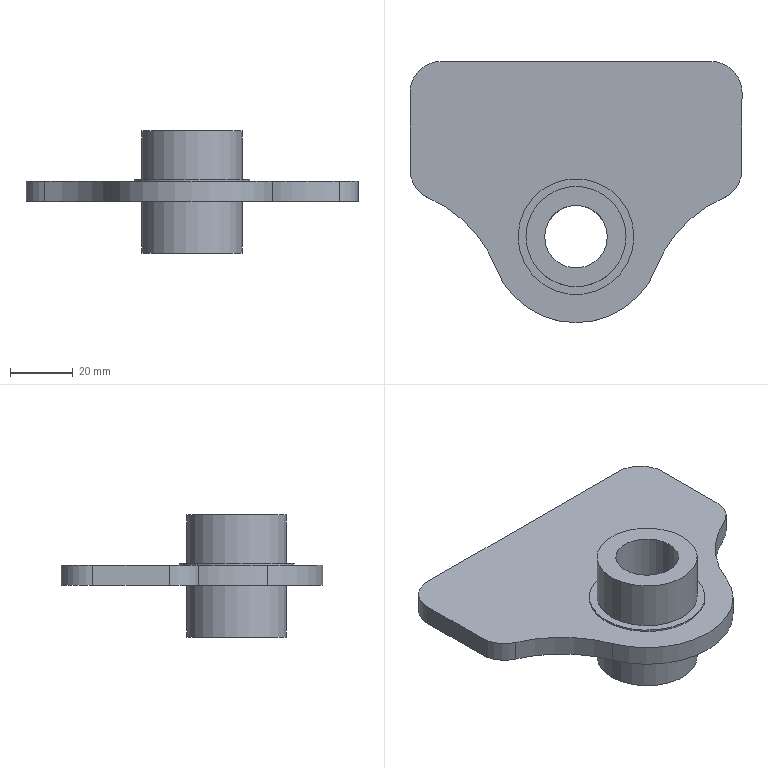NC program | NX | posted with a generic post | part box 106 x 83.448 x 39 mm
Lines 1987 to 2052 of 2052:
(PLANAR_MILL_4_COPY , TOOL : D16-48-D16-100-3T-FINISH)
N3942 T03 M6
N3944 G53
N3946 G17 G0 G90 X0.197 Y0.965 S3000 M3
N3948 G43 Z30. H3
N3950 Z-37.
N3952 G94 G1 Z-39. F300.
N3954 G41 X0. Y1. D3
N3956 X-1.
N3958 G3 X-2. Y0. R1.
N3960 X0. Y-2. R2.
N3962 X-2. Y0. R-2.
N3964 X-1. Y-1. R1.
N3966 G40
N3968 G1 X-0.803 Y-0.965
N3970 Y0.965
N3972 G41 X-1. Y1.
N3974 G3 X-2. Y0. R1.
N3976 X0. Y-2. R2.
N3978 X-2. Y0. R-2.
N3980 X-1. Y-1. R1.
N3982 G1 X0.
N3984 G40
N3986 X0.197 Y-0.965
N3988 Z-37.
N3990 G0 Z30.
N3992 M5
(PLANAR_MILL_3 , TOOL : CHAMFER_D6-90DEG)
N3994 T02 M6
N3996 G53
N3998 G17 G0 G90 X-19.992 Y-1.913 S3000 M3
N4000 G43 Z30. H2
N4002 Z0.
N4004 G94 G1 Z-2. F600.
N4006 G41 X-19.5 Y-2. D2
N4008 G3 X-17.5 Y0. R2.
N4010 G2 X0. Y17.5 R17.5
N4012 X-17.5 Y0. R-17.5
N4014 G3 X-19.5 Y2. R2.
N4016 G40
N4018 G1 X-19.992 Y1.913
N4020 Z0.
N4022 G0 Z30.
(PLANAR_MILL_3_COPY , TOOL : CHAMFER_D6-90DEG)
N4024 X-5.692
N4026 Z0.
N4028 G1 Z-2.
N4030 G41 X-6.185 Y2.
N4032 X-6.5
N4034 G3 X-8.5 Y0. R2.
N4036 X0. Y-8.5 R8.5
N4038 X-8.5 Y0. R-8.5
N4040 X-6.5 Y-2. R2.
N4042 G1 X-6.185
N4044 G40
N4046 X-5.692 Y-1.913
N4048 Z0.
N4050 G0 Z30.
N4052 M5
N4054 M2